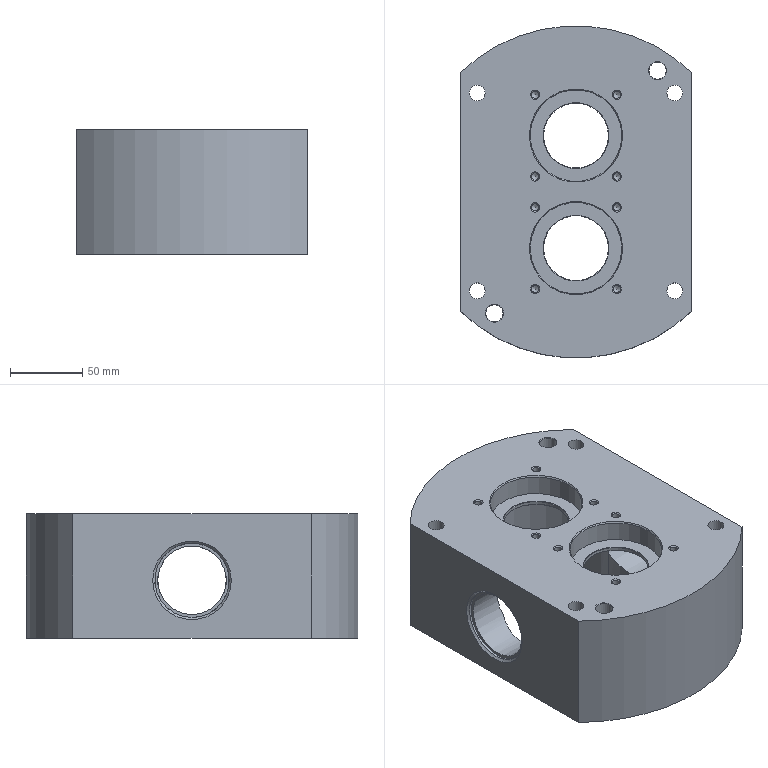NC program | NX | posted with a generic post | part box 160 x 230 x 86 mm
Lines 2291 to 2342 of 2342:
(PLANAR_MILL , TOOL : D6A45)
N4550 T07 M6
N4552 G54
N4554 G17 G0 G90 X84.087 Y-44.7 B0. C0. S7500 M3
N4556 G43 Z30. H7
N4558 Z-33.
N4560 G94 G1 Z-36. F1250.
N4562 X83.38 Y-43.857
N4564 G3 X82.614 Y-43.5 R1.
N4566 G1 X-82.614
N4568 G3 X-83.38 Y-43.857 R1.
N4570 G1 X-84.087 Y-44.7
N4572 Z-33.
N4574 G0 Z30.
N4576 Y44.7
N4578 Z-33.
N4580 G1 Z-36.
N4582 X-83.38 Y43.857
N4584 G3 X-82.614 Y43.5 R1.
N4586 G1 X82.614
N4588 G3 X83.38 Y43.857 R1.
N4590 G1 X84.087 Y44.7
N4592 Z-33.
N4594 G0 Z30.
(PLANAR_MILL_COPY , TOOL : D6A45)
N4596 X1.515 Y20.
N4598 Z-34.
N4600 G1 Z-37.
N4602 X0.766 Y20.893
N4604 G3 X0. Y21.25 R1.
N4606 X-24.25 Y-3. R24.25
N4608 X0. Y21.25 R-24.25
N4610 X-0.766 Y20.893 R1.
N4612 G1 X0.766 Y21.393
N4614 G3 X0. Y21.75 R1.
N4616 X-24.75 Y-3. R24.75
N4618 X0. Y21.75 R-24.75
N4620 X-0.766 Y21.393 R1.
N4622 G1 X0.766 Y21.893
N4624 G3 X0. Y22.25 R1.
N4626 X-25.25 Y-3. R25.25
N4628 X0. Y22.25 R-25.25
N4630 X-0.766 Y21.893 R1.
N4632 G1 X-1.513 Y21.002
N4634 Z-34.
N4636 G0 Z30.
N4638 M5
N4640 M2